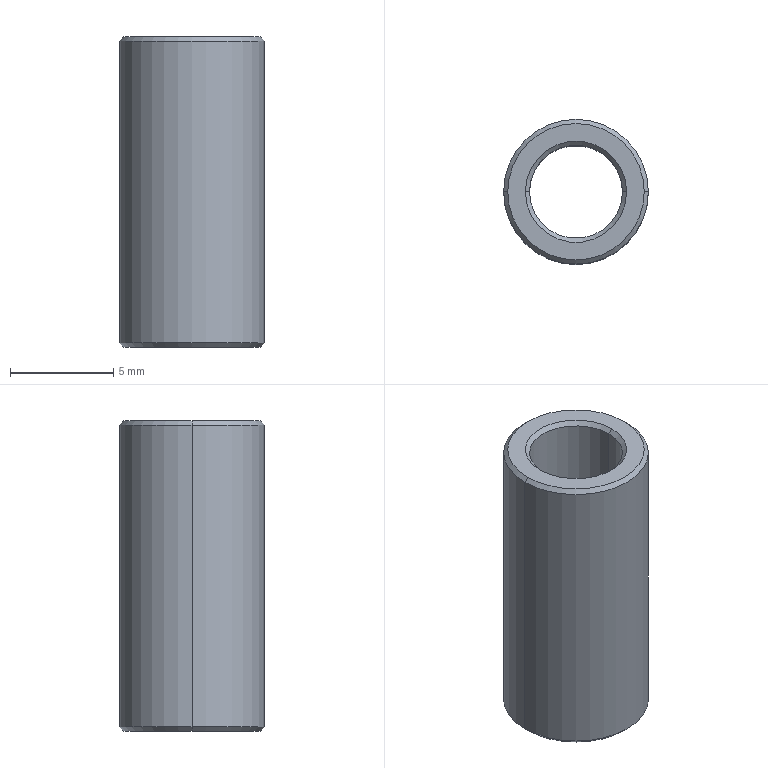Part | SolidWorks | features Chamfer 1, Extrusion 1 | 1 solid | 14 faces | box 7 x 7 x 15 mm | volume 337.258 mm3 | cone 8 | cylinder 4 | plane 2 | commonest cylinder face diameters 4.5 x2 7 x2
STEP:
#1=CARTESIAN_POINT('',(3.3,0.,7.5));
#2=VERTEX_POINT('',#1);
#3=CARTESIAN_POINT('',(-3.3,0.,7.5));
#4=VERTEX_POINT('',#3);
#5=CARTESIAN_POINT('',(0.,0.,7.5));
#6=DIRECTION('',(0.,0.,1.));
#7=DIRECTION('',(1.,0.,0.));
#8=AXIS2_PLACEMENT_3D('',#5,#6,#7);
#9=CIRCLE('',#8,3.3);
#10=EDGE_CURVE('',#2,#4,#9,.T.);
#11=ORIENTED_EDGE('',*,*,#10,.F.);
#12=CARTESIAN_POINT('',(3.5,0.,7.3));
#13=VERTEX_POINT('',#12);
#14=CARTESIAN_POINT('',(3.3,0.,7.5));
#15=DIRECTION('',(0.7071,0.,-0.7071));
#16=VECTOR('',#15,1000.);
#17=LINE('',#14,#16);
#18=EDGE_CURVE('',#2,#13,#17,.T.);
#19=ORIENTED_EDGE('',*,*,#18,.T.);
#20=CARTESIAN_POINT('',(-3.5,0.,7.3));
#21=VERTEX_POINT('',#20);
#22=CARTESIAN_POINT('',(0.,0.,7.3));
#23=DIRECTION('',(0.,0.,-1.));
#24=DIRECTION('',(1.,0.,0.));
#25=AXIS2_PLACEMENT_3D('',#22,#23,#24);
#26=CIRCLE('',#25,3.5);
#27=EDGE_CURVE('',#21,#13,#26,.T.);
#28=ORIENTED_EDGE('',*,*,#27,.F.);
#29=CARTESIAN_POINT('',(-3.3,0.,7.5));
#30=DIRECTION('',(-0.7071,0.,-0.7071));
#31=VECTOR('',#30,1000.);
#32=LINE('',#29,#31);
#33=EDGE_CURVE('',#4,#21,#32,.T.);
#34=ORIENTED_EDGE('',*,*,#33,.F.);
#35=EDGE_LOOP('',(#11,#19,#28,#34));
#36=FACE_OUTER_BOUND('',#35,.T.);
#37=CARTESIAN_POINT('',(0.,0.,7.5));
#38=DIRECTION('',(0.,0.,-1.));
#39=DIRECTION('',(-1.,0.,0.));
#40=AXIS2_PLACEMENT_3D('',#37,#38,#39);
#41=CONICAL_SURFACE('',#40,3.3,0.7854);
#42=ADVANCED_FACE('',(#36),#41,.T.);
#43=CARTESIAN_POINT('',(-2.25,0.,7.3));
#44=VERTEX_POINT('',#43);
#45=CARTESIAN_POINT('',(2.25,0.,7.3));
#46=VERTEX_POINT('',#45);
#47=CARTESIAN_POINT('',(0.,0.,7.3));
#48=DIRECTION('',(0.,0.,1.));
#49=DIRECTION('',(1.,0.,0.));
#50=AXIS2_PLACEMENT_3D('',#47,#48,#49);
#51=CIRCLE('',#50,2.25);
#52=EDGE_CURVE('',#44,#46,#51,.T.);
#53=ORIENTED_EDGE('',*,*,#52,.F.);
#54=CARTESIAN_POINT('',(-2.45,0.,7.5));
#55=VERTEX_POINT('',#54);
#56=CARTESIAN_POINT('',(-2.25,0.,7.3));
#57=DIRECTION('',(-0.7071,0.,0.7071));
#58=VECTOR('',#57,1000.);
#59=LINE('',#56,#58);
#60=EDGE_CURVE('',#44,#55,#59,.T.);
#61=ORIENTED_EDGE('',*,*,#60,.T.);
#62=CARTESIAN_POINT('',(2.45,0.,7.5));
#63=VERTEX_POINT('',#62);
#64=CARTESIAN_POINT('',(0.,0.,7.5));
#65=DIRECTION('',(0.,0.,-1.));
#66=DIRECTION('',(1.,0.,0.));
#67=AXIS2_PLACEMENT_3D('',#64,#65,#66);
#68=CIRCLE('',#67,2.45);
#69=EDGE_CURVE('',#63,#55,#68,.T.);
#70=ORIENTED_EDGE('',*,*,#69,.F.);
#71=CARTESIAN_POINT('',(2.25,0.,7.3));
#72=DIRECTION('',(0.7071,0.,0.7071));
#73=VECTOR('',#72,1000.);
#74=LINE('',#71,#73);
#75=EDGE_CURVE('',#46,#63,#74,.T.);
#76=ORIENTED_EDGE('',*,*,#75,.F.);
#77=EDGE_LOOP('',(#53,#61,#70,#76));
#78=FACE_OUTER_BOUND('',#77,.T.);
#79=CARTESIAN_POINT('',(0.,0.,7.3));
#80=DIRECTION('',(0.,0.,1.));
#81=DIRECTION('',(1.,0.,0.));
#82=AXIS2_PLACEMENT_3D('',#79,#80,#81);
#83=CONICAL_SURFACE('',#82,2.25,0.7854);
#84=ADVANCED_FACE('',(#78),#83,.F.);
#85=CARTESIAN_POINT('',(-3.3,0.,-7.5));
#86=VERTEX_POINT('',#85);
#87=CARTESIAN_POINT('',(3.3,0.,-7.5));
#88=VERTEX_POINT('',#87);
#89=CARTESIAN_POINT('',(0.,0.,-7.5));
#90=DIRECTION('',(0.,0.,-1.));
#91=DIRECTION('',(1.,0.,0.));
#92=AXIS2_PLACEMENT_3D('',#89,#90,#91);
#93=CIRCLE('',#92,3.3);
#94=EDGE_CURVE('',#86,#88,#93,.T.);
#95=ORIENTED_EDGE('',*,*,#94,.F.);
#96=CARTESIAN_POINT('',(-3.5,0.,-7.3));
#97=VERTEX_POINT('',#96);
#98=CARTESIAN_POINT('',(-3.5,0.,-7.3));
#99=DIRECTION('',(-0.7071,0.,0.7071));
#100=VECTOR('',#99,1000.);
#101=LINE('',#98,#100);
#102=EDGE_CURVE('',#86,#97,#101,.T.);
#103=ORIENTED_EDGE('',*,*,#102,.T.);
#104=CARTESIAN_POINT('',(3.5,0.,-7.3));
#105=VERTEX_POINT('',#104);
#106=CARTESIAN_POINT('',(0.,0.,-7.3));
#107=DIRECTION('',(0.,0.,1.));
#108=DIRECTION('',(1.,0.,0.));
#109=AXIS2_PLACEMENT_3D('',#106,#107,#108);
#110=CIRCLE('',#109,3.5);
#111=EDGE_CURVE('',#105,#97,#110,.T.);
#112=ORIENTED_EDGE('',*,*,#111,.F.);
#113=CARTESIAN_POINT('',(3.5,0.,-7.3));
#114=DIRECTION('',(0.7071,0.,0.7071));
#115=VECTOR('',#114,1000.);
#116=LINE('',#113,#115);
#117=EDGE_CURVE('',#88,#105,#116,.T.);
#118=ORIENTED_EDGE('',*,*,#117,.F.);
#119=EDGE_LOOP('',(#95,#103,#112,#118));
#120=FACE_OUTER_BOUND('',#119,.T.);
#121=CARTESIAN_POINT('',(0.,0.,-7.3));
#122=DIRECTION('',(0.,0.,1.));
#123=DIRECTION('',(1.,0.,0.));
#124=AXIS2_PLACEMENT_3D('',#121,#122,#123);
#125=CONICAL_SURFACE('',#124,3.5,0.7854);
#126=ADVANCED_FACE('',(#120),#125,.T.);
#127=CARTESIAN_POINT('',(2.25,0.,-7.3));
#128=VERTEX_POINT('',#127);
#129=CARTESIAN_POINT('',(-2.25,0.,-7.3));
#130=VERTEX_POINT('',#129);
#131=CARTESIAN_POINT('',(0.,0.,-7.3));
#132=DIRECTION('',(0.,0.,-1.));
#133=DIRECTION('',(1.,0.,0.));
#134=AXIS2_PLACEMENT_3D('',#131,#132,#133);
#135=CIRCLE('',#134,2.25);
#136=EDGE_CURVE('',#128,#130,#135,.T.);
#137=ORIENTED_EDGE('',*,*,#136,.F.);
#138=CARTESIAN_POINT('',(2.45,0.,-7.5));
#139=VERTEX_POINT('',#138);
#140=CARTESIAN_POINT('',(2.45,0.,-7.5));
#141=DIRECTION('',(0.7071,0.,-0.7071));
#142=VECTOR('',#141,1000.);
#143=LINE('',#140,#142);
#144=EDGE_CURVE('',#128,#139,#143,.T.);
#145=ORIENTED_EDGE('',*,*,#144,.T.);
#146=CARTESIAN_POINT('',(-2.45,0.,-7.5));
#147=VERTEX_POINT('',#146);
#148=CARTESIAN_POINT('',(0.,0.,-7.5));
#149=DIRECTION('',(0.,0.,1.));
#150=DIRECTION('',(1.,0.,0.));
#151=AXIS2_PLACEMENT_3D('',#148,#149,#150);
#152=CIRCLE('',#151,2.45);
#153=EDGE_CURVE('',#147,#139,#152,.T.);
#154=ORIENTED_EDGE('',*,*,#153,.F.);
#155=CARTESIAN_POINT('',(-2.45,0.,-7.5));
#156=DIRECTION('',(-0.7071,0.,-0.7071));
#157=VECTOR('',#156,1000.);
#158=LINE('',#155,#157);
#159=EDGE_CURVE('',#130,#147,#158,.T.);
#160=ORIENTED_EDGE('',*,*,#159,.F.);
#161=EDGE_LOOP('',(#137,#145,#154,#160));
#162=FACE_OUTER_BOUND('',#161,.T.);
#163=CARTESIAN_POINT('',(0.,0.,-7.5));
#164=DIRECTION('',(0.,0.,-1.));
#165=DIRECTION('',(-1.,0.,0.));
#166=AXIS2_PLACEMENT_3D('',#163,#164,#165);
#167=CONICAL_SURFACE('',#166,2.45,0.7854);
#168=ADVANCED_FACE('',(#162),#167,.F.);
#169=ORIENTED_EDGE('',*,*,#52,.T.);
#170=CARTESIAN_POINT('',(2.25,0.,7.5));
#171=DIRECTION('',(0.,0.,-1.));
#172=VECTOR('',#171,1000.);
#173=LINE('',#170,#172);
#174=EDGE_CURVE('',#46,#128,#173,.T.);
#175=ORIENTED_EDGE('',*,*,#174,.T.);
#176=ORIENTED_EDGE('',*,*,#136,.T.);
#177=CARTESIAN_POINT('',(-2.25,0.,7.5));
#178=DIRECTION('',(0.,0.,-1.));
#179=VECTOR('',#178,1000.);
#180=LINE('',#177,#179);
#181=EDGE_CURVE('',#44,#130,#180,.T.);
#182=ORIENTED_EDGE('',*,*,#181,.F.);
#183=EDGE_LOOP('',(#169,#175,#176,#182));
#184=FACE_OUTER_BOUND('',#183,.T.);
#185=CARTESIAN_POINT('',(0.,0.,7.5));
#186=DIRECTION('',(0.,0.,-1.));
#187=DIRECTION('',(-1.,0.,0.));
#188=AXIS2_PLACEMENT_3D('',#185,#186,#187);
#189=CYLINDRICAL_SURFACE('',#188,2.25);
#190=ADVANCED_FACE('',(#184),#189,.F.);
#191=ORIENTED_EDGE('',*,*,#27,.T.);
#192=CARTESIAN_POINT('',(3.5,0.,7.5));
#193=DIRECTION('',(0.,0.,-1.));
#194=VECTOR('',#193,1000.);
#195=LINE('',#192,#194);
#196=EDGE_CURVE('',#13,#105,#195,.T.);
#197=ORIENTED_EDGE('',*,*,#196,.T.);
#198=ORIENTED_EDGE('',*,*,#111,.T.);
#199=CARTESIAN_POINT('',(-3.5,0.,7.5));
#200=DIRECTION('',(0.,0.,-1.));
#201=VECTOR('',#200,1000.);
#202=LINE('',#199,#201);
#203=EDGE_CURVE('',#21,#97,#202,.T.);
#204=ORIENTED_EDGE('',*,*,#203,.F.);
#205=EDGE_LOOP('',(#191,#197,#198,#204));
#206=FACE_OUTER_BOUND('',#205,.T.);
#207=CARTESIAN_POINT('',(0.,0.,7.5));
#208=DIRECTION('',(0.,0.,-1.));
#209=DIRECTION('',(-1.,0.,0.));
#210=AXIS2_PLACEMENT_3D('',#207,#208,#209);
#211=CYLINDRICAL_SURFACE('',#210,3.5);
#212=ADVANCED_FACE('',(#206),#211,.T.);
#213=ORIENTED_EDGE('',*,*,#69,.T.);
#214=CARTESIAN_POINT('',(0.,0.,7.5));
#215=DIRECTION('',(0.,0.,-1.));
#216=DIRECTION('',(1.,0.,0.));
#217=AXIS2_PLACEMENT_3D('',#214,#215,#216);
#218=CIRCLE('',#217,2.45);
#219=EDGE_CURVE('',#55,#63,#218,.T.);
#220=ORIENTED_EDGE('',*,*,#219,.T.);
#221=EDGE_LOOP('',(#213,#220));
#222=FACE_BOUND('',#221,.T.);
#223=CARTESIAN_POINT('',(0.,0.,7.5));
#224=DIRECTION('',(0.,0.,1.));
#225=DIRECTION('',(1.,0.,0.));
#226=AXIS2_PLACEMENT_3D('',#223,#224,#225);
#227=CIRCLE('',#226,3.3);
#228=EDGE_CURVE('',#4,#2,#227,.T.);
#229=ORIENTED_EDGE('',*,*,#228,.T.);
#230=ORIENTED_EDGE('',*,*,#10,.T.);
#231=EDGE_LOOP('',(#229,#230));
#232=FACE_OUTER_BOUND('',#231,.T.);
#233=CARTESIAN_POINT('',(0.,0.,7.5));
#234=DIRECTION('',(0.,0.,1.));
#235=DIRECTION('',(1.,0.,0.));
#236=AXIS2_PLACEMENT_3D('',#233,#234,#235);
#237=PLANE('',#236);
#238=ADVANCED_FACE('',(#222,#232),#237,.T.);
#239=ORIENTED_EDGE('',*,*,#153,.T.);
#240=CARTESIAN_POINT('',(0.,0.,-7.5));
#241=DIRECTION('',(0.,0.,1.));
#242=DIRECTION('',(1.,0.,0.));
#243=AXIS2_PLACEMENT_3D('',#240,#241,#242);
#244=CIRCLE('',#243,2.45);
#245=EDGE_CURVE('',#139,#147,#244,.T.);
#246=ORIENTED_EDGE('',*,*,#245,.T.);
#247=EDGE_LOOP('',(#239,#246));
#248=FACE_BOUND('',#247,.T.);
#249=CARTESIAN_POINT('',(0.,0.,-7.5));
#250=DIRECTION('',(0.,0.,-1.));
#251=DIRECTION('',(1.,0.,0.));
#252=AXIS2_PLACEMENT_3D('',#249,#250,#251);
#253=CIRCLE('',#252,3.3);
#254=EDGE_CURVE('',#88,#86,#253,.T.);
#255=ORIENTED_EDGE('',*,*,#254,.T.);
#256=ORIENTED_EDGE('',*,*,#94,.T.);
#257=EDGE_LOOP('',(#255,#256));
#258=FACE_OUTER_BOUND('',#257,.T.);
#259=CARTESIAN_POINT('',(0.,0.,-7.5));
#260=DIRECTION('',(0.,0.,1.));
#261=DIRECTION('',(1.,0.,0.));
#262=AXIS2_PLACEMENT_3D('',#259,#260,#261);
#263=PLANE('',#262);
#264=ADVANCED_FACE('',(#248,#258),#263,.F.);
#265=ORIENTED_EDGE('',*,*,#196,.F.);
#266=CARTESIAN_POINT('',(0.,0.,7.3));
#267=DIRECTION('',(0.,0.,-1.));
#268=DIRECTION('',(1.,0.,0.));
#269=AXIS2_PLACEMENT_3D('',#266,#267,#268);
#270=CIRCLE('',#269,3.5);
#271=EDGE_CURVE('',#13,#21,#270,.T.);
#272=ORIENTED_EDGE('',*,*,#271,.T.);
#273=ORIENTED_EDGE('',*,*,#203,.T.);
#274=CARTESIAN_POINT('',(0.,0.,-7.3));
#275=DIRECTION('',(0.,0.,1.));
#276=DIRECTION('',(1.,0.,0.));
#277=AXIS2_PLACEMENT_3D('',#274,#275,#276);
#278=CIRCLE('',#277,3.5);
#279=EDGE_CURVE('',#97,#105,#278,.T.);
#280=ORIENTED_EDGE('',*,*,#279,.T.);
#281=EDGE_LOOP('',(#265,#272,#273,#280));
#282=FACE_OUTER_BOUND('',#281,.T.);
#283=CARTESIAN_POINT('',(0.,0.,7.5));
#284=DIRECTION('',(0.,0.,-1.));
#285=DIRECTION('',(-1.,0.,0.));
#286=AXIS2_PLACEMENT_3D('',#283,#284,#285);
#287=CYLINDRICAL_SURFACE('',#286,3.5);
#288=ADVANCED_FACE('',(#282),#287,.T.);
#289=ORIENTED_EDGE('',*,*,#174,.F.);
#290=CARTESIAN_POINT('',(0.,0.,7.3));
#291=DIRECTION('',(0.,0.,1.));
#292=DIRECTION('',(1.,0.,0.));
#293=AXIS2_PLACEMENT_3D('',#290,#291,#292);
#294=CIRCLE('',#293,2.25);
#295=EDGE_CURVE('',#46,#44,#294,.T.);
#296=ORIENTED_EDGE('',*,*,#295,.T.);
#297=ORIENTED_EDGE('',*,*,#181,.T.);
#298=CARTESIAN_POINT('',(0.,0.,-7.3));
#299=DIRECTION('',(0.,0.,-1.));
#300=DIRECTION('',(1.,0.,0.));
#301=AXIS2_PLACEMENT_3D('',#298,#299,#300);
#302=CIRCLE('',#301,2.25);
#303=EDGE_CURVE('',#130,#128,#302,.T.);
#304=ORIENTED_EDGE('',*,*,#303,.T.);
#305=EDGE_LOOP('',(#289,#296,#297,#304));
#306=FACE_OUTER_BOUND('',#305,.T.);
#307=CARTESIAN_POINT('',(0.,0.,7.5));
#308=DIRECTION('',(0.,0.,-1.));
#309=DIRECTION('',(-1.,0.,0.));
#310=AXIS2_PLACEMENT_3D('',#307,#308,#309);
#311=CYLINDRICAL_SURFACE('',#310,2.25);
#312=ADVANCED_FACE('',(#306),#311,.F.);
#313=ORIENTED_EDGE('',*,*,#144,.F.);
#314=ORIENTED_EDGE('',*,*,#303,.F.);
#315=ORIENTED_EDGE('',*,*,#159,.T.);
#316=ORIENTED_EDGE('',*,*,#245,.F.);
#317=EDGE_LOOP('',(#313,#314,#315,#316));
#318=FACE_OUTER_BOUND('',#317,.T.);
#319=CARTESIAN_POINT('',(0.,0.,-7.5));
#320=DIRECTION('',(0.,0.,-1.));
#321=DIRECTION('',(-1.,0.,0.));
#322=AXIS2_PLACEMENT_3D('',#319,#320,#321);
#323=CONICAL_SURFACE('',#322,2.45,0.7854);
#324=ADVANCED_FACE('',(#318),#323,.F.);
#325=ORIENTED_EDGE('',*,*,#102,.F.);
#326=ORIENTED_EDGE('',*,*,#254,.F.);
#327=ORIENTED_EDGE('',*,*,#117,.T.);
#328=ORIENTED_EDGE('',*,*,#279,.F.);
#329=EDGE_LOOP('',(#325,#326,#327,#328));
#330=FACE_OUTER_BOUND('',#329,.T.);
#331=CARTESIAN_POINT('',(0.,0.,-7.3));
#332=DIRECTION('',(0.,0.,1.));
#333=DIRECTION('',(1.,0.,0.));
#334=AXIS2_PLACEMENT_3D('',#331,#332,#333);
#335=CONICAL_SURFACE('',#334,3.5,0.7854);
#336=ADVANCED_FACE('',(#330),#335,.T.);
#337=ORIENTED_EDGE('',*,*,#60,.F.);
#338=ORIENTED_EDGE('',*,*,#295,.F.);
#339=ORIENTED_EDGE('',*,*,#75,.T.);
#340=ORIENTED_EDGE('',*,*,#219,.F.);
#341=EDGE_LOOP('',(#337,#338,#339,#340));
#342=FACE_OUTER_BOUND('',#341,.T.);
#343=CARTESIAN_POINT('',(0.,0.,7.3));
#344=DIRECTION('',(0.,0.,1.));
#345=DIRECTION('',(1.,0.,0.));
#346=AXIS2_PLACEMENT_3D('',#343,#344,#345);
#347=CONICAL_SURFACE('',#346,2.25,0.7854);
#348=ADVANCED_FACE('',(#342),#347,.F.);
#349=ORIENTED_EDGE('',*,*,#18,.F.);
#350=ORIENTED_EDGE('',*,*,#228,.F.);
#351=ORIENTED_EDGE('',*,*,#33,.T.);
#352=ORIENTED_EDGE('',*,*,#271,.F.);
#353=EDGE_LOOP('',(#349,#350,#351,#352));
#354=FACE_OUTER_BOUND('',#353,.T.);
#355=CARTESIAN_POINT('',(0.,0.,7.5));
#356=DIRECTION('',(0.,0.,-1.));
#357=DIRECTION('',(-1.,0.,0.));
#358=AXIS2_PLACEMENT_3D('',#355,#356,#357);
#359=CONICAL_SURFACE('',#358,3.3,0.7854);
#360=ADVANCED_FACE('',(#354),#359,.T.);
#361=CLOSED_SHELL('',(#42,#84,#126,#168,#190,#212,#238,#264,#288,#312,#324,#336,#348,#360));
#362=MANIFOLD_SOLID_BREP('',#361);
#363=CARTESIAN_POINT('',(0.,0.,0.));
#364=DIRECTION('',(0.,0.,1.));
#365=DIRECTION('',(1.,0.,0.));
#366=AXIS2_PLACEMENT_3D('',#363,#364,#365);
#367=(LENGTH_UNIT()NAMED_UNIT(*)SI_UNIT(.MILLI.,.METRE.));
#368=UNCERTAINTY_MEASURE_WITH_UNIT(LENGTH_MEASURE(0.00001),#367,'','');
#369=(NAMED_UNIT(*)PLANE_ANGLE_UNIT()SI_UNIT($,.RADIAN.));
#370=(NAMED_UNIT(*)SI_UNIT($,.STERADIAN.)SOLID_ANGLE_UNIT());
#371=(GEOMETRIC_REPRESENTATION_CONTEXT(3)GLOBAL_UNCERTAINTY_ASSIGNED_CONTEXT((#368))GLOBAL_UNIT_ASSIGNED_CONTEXT((#367,#369,#370))REPRESENTATION_CONTEXT('',''));
#372=ADVANCED_BREP_SHAPE_REPRESENTATION('',(#362,#366),#371);